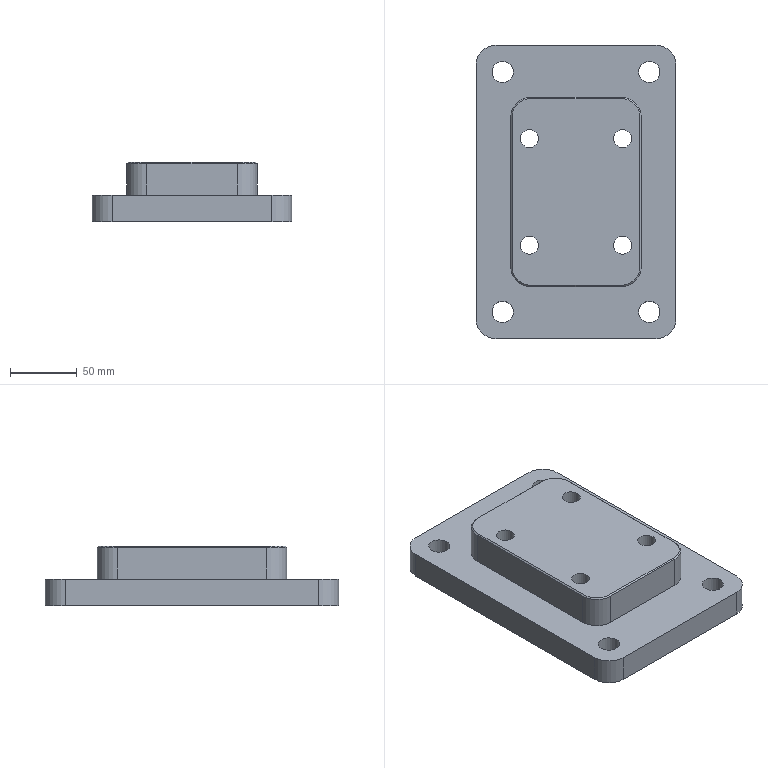NC program | NX | posted with a generic post | part box 150 x 220 x 45 mm
Lines 40 to 1292 of 5916:
(ZLEVEL_PROFILE_1_COPY , TOOL : D10)
N72 T10 M6
N74 G54
N76 G17 G0 G90 X91.61 Y82.1 S3200 M3
N78 G43 Z30. H10
N80 Z1.78
N82 G94 G1 Z-0.22 F2200.
N84 X92.478 Y80.599
N86 G3 X93.345 Y80.099 R1.
N88 G1 X94.677 Y80.1
N90 X95.
N92 G2 X115.1 Y60. R20.1
N94 G1 Y59.677
N96 Y58.345
N98 G3 X115.6 Y57.479 R1.
N100 G1 X117.1 Y56.612
N102 Z1.78
N104 G0 Z30.
N106 Z1.56
N108 G1 Z-0.44
N110 X115.6 Y57.479
N112 G2 X115.1 Y58.345 R1.
N114 G1 Y59.677
N116 Y60.
N118 G3 X95. Y80.1 R20.1
N120 G1 X94.677
N122 X93.345 Y80.099
N124 G2 X92.478 Y80.599 R1.
N126 G1 X91.61 Y82.1
N128 Z1.56
N130 G0 Z30.
N132 Z1.341
N134 G1 Z-0.659
N136 X92.478 Y80.599
N138 G3 X93.345 Y80.099 R1.
N140 G1 X94.677 Y80.1
N142 X95.
N144 G2 X115.1 Y60. R20.1
N146 G1 Y59.677
N148 Y58.345
N150 G3 X115.6 Y57.479 R1.
N152 G1 X117.1 Y56.612
N154 Z1.341
N156 G0 Z30.
N158 Z1.121
N160 G1 Z-0.879
N162 X115.6 Y57.479
N164 G2 X115.1 Y58.345 R1.
N166 G1 Y59.677
N168 Y60.
N170 G3 X95. Y80.1 R20.1
N172 G1 X94.677
N174 X93.345 Y80.099
N176 G2 X92.478 Y80.599 R1.
N178 G1 X91.61 Y82.1
N180 Z1.121
N182 G0 Z30.
N184 Z0.901
N186 G1 Z-1.099
N188 X92.478 Y80.599
N190 G3 X93.345 Y80.099 R1.
N192 G1 X94.677 Y80.1
N194 X95.
N196 G2 X115.1 Y60. R20.1
N198 G1 Y59.677
N200 Y58.345
N202 G3 X115.6 Y57.479 R1.
N204 G1 X117.1 Y56.612
N206 Z0.901
N208 G0 Z30.
N210 Z0.681
N212 G1 Z-1.319
N214 X115.6 Y57.479
N216 G2 X115.1 Y58.345 R1.
N218 G1 Y59.677
N220 Y60.
N222 G3 X95. Y80.1 R20.1
N224 G1 X94.677
N226 X93.345 Y80.099
N228 G2 X92.478 Y80.599 R1.
N230 G1 X91.61 Y82.1
N232 Z0.681
N234 G0 Z30.
N236 Z0.462
N238 G1 Z-1.538
N240 X92.478 Y80.599
N242 G3 X93.345 Y80.099 R1.
N244 G1 X94.677 Y80.1
N246 X95.
N248 G2 X115.1 Y60. R20.1
N250 G1 Y59.677
N252 Y58.345
N254 G3 X115.6 Y57.479 R1.
N256 G1 X117.1 Y56.612
N258 Z0.462
N260 G0 Z30.
N262 Z0.242
N264 G1 Z-1.758
N266 X115.6 Y57.479
N268 G2 X115.1 Y58.345 R1.
N270 G1 Y59.677
N272 Y60.
N274 G3 X95. Y80.1 R20.1
N276 G1 X94.677
N278 X93.345 Y80.099
N280 G2 X92.478 Y80.599 R1.
N282 G1 X91.61 Y82.1
N284 Z0.242
N286 G0 Z30.
N288 Z0.022
N290 G1 Z-1.978
N292 X92.478 Y80.599
N294 G3 X93.345 Y80.099 R1.
N296 G1 X94.677 Y80.1
N298 X95.
N300 G2 X115.1 Y60. R20.1
N302 G1 Y59.677
N304 Y58.345
N306 G3 X115.6 Y57.479 R1.
N308 G1 X117.1 Y56.612
N310 Z0.022
N312 G0 Z30.
N314 Z-0.198
N316 G1 Z-2.198
N318 X115.6 Y57.479
N320 G2 X115.1 Y58.345 R1.
N322 G1 Y59.677
N324 Y60.
N326 G3 X95. Y80.1 R20.1
N328 G1 X94.677
N330 X93.345 Y80.099
N332 G2 X92.478 Y80.599 R1.
N334 G1 X91.61 Y82.1
N336 Z-0.198
N338 G0 Z30.
N340 Z-0.418
N342 G1 Z-2.418
N344 X92.478 Y80.599
N346 G3 X93.345 Y80.099 R1.
N348 G1 X94.677 Y80.1
N350 X95.
N352 G2 X115.1 Y60. R20.1
N354 G1 Y59.677
N356 Y58.345
N358 G3 X115.6 Y57.479 R1.
N360 G1 X117.1 Y56.612
N362 Z-0.418
N364 G0 Z30.
N366 Z-0.637
N368 G1 Z-2.637
N370 X115.6 Y57.479
N372 G2 X115.1 Y58.345 R1.
N374 G1 Y59.677
N376 Y60.
N378 G3 X95. Y80.1 R20.1
N380 G1 X94.677
N382 X93.345 Y80.099
N384 G2 X92.478 Y80.599 R1.
N386 G1 X91.61 Y82.1
N388 Z-0.637
N390 G0 Z30.
N392 Z-0.857
N394 G1 Z-2.857
N396 X92.478 Y80.599
N398 G3 X93.345 Y80.099 R1.
N400 G1 X94.677 Y80.1
N402 X95.
N404 G2 X115.1 Y60. R20.1
N406 G1 Y59.677
N408 Y58.345
N410 G3 X115.6 Y57.479 R1.
N412 G1 X117.1 Y56.612
N414 Z-0.857
N416 G0 Z30.
N418 Z-1.077
N420 G1 Z-3.077
N422 X115.6 Y57.479
N424 G2 X115.1 Y58.345 R1.
N426 G1 Y59.677
N428 Y60.
N430 G3 X95. Y80.1 R20.1
N432 G1 X94.677
N434 X93.345 Y80.099
N436 G2 X92.478 Y80.599 R1.
N438 G1 X91.61 Y82.1
N440 Z-1.077
N442 G0 Z30.
N444 Z-1.297
N446 G1 Z-3.297
N448 X92.478 Y80.599
N450 G3 X93.345 Y80.099 R1.
N452 G1 X94.677 Y80.1
N454 X95.
N456 G2 X115.1 Y60. R20.1
N458 G1 Y59.677
N460 Y58.345
N462 G3 X115.6 Y57.479 R1.
N464 G1 X117.1 Y56.612
N466 Z-1.297
N468 G0 Z30.
N470 Z-1.516
N472 G1 Z-3.516
N474 X115.6 Y57.479
N476 G2 X115.1 Y58.345 R1.
N478 G1 Y59.677
N480 Y60.
N482 G3 X95. Y80.1 R20.1
N484 G1 X94.677
N486 X93.345 Y80.099
N488 G2 X92.478 Y80.599 R1.
N490 G1 X91.61 Y82.1
N492 Z-1.516
N494 G0 Z30.
N496 Z-1.736
N498 G1 Z-3.736
N500 X92.478 Y80.599
N502 G3 X93.345 Y80.099 R1.
N504 G1 X94.677 Y80.1
N506 X95.
N508 G2 X115.1 Y60. R20.1
N510 G1 Y59.677
N512 Y58.345
N514 G3 X115.6 Y57.479 R1.
N516 G1 X117.1 Y56.612
N518 Z-1.736
N520 G0 Z30.
N522 Z-1.956
N524 G1 Z-3.956
N526 X115.6 Y57.479
N528 G2 X115.1 Y58.345 R1.
N530 G1 Y59.677
N532 Y60.
N534 G3 X95. Y80.1 R20.1
N536 G1 X94.677
N538 X93.345 Y80.099
N540 G2 X92.478 Y80.599 R1.
N542 G1 X91.61 Y82.1
N544 Z-1.956
N546 G0 Z30.
N548 Z-2.176
N550 G1 Z-4.176
N552 X92.478 Y80.599
N554 G3 X93.345 Y80.099 R1.
N556 G1 X94.677 Y80.1
N558 X95.
N560 G2 X115.1 Y60. R20.1
N562 G1 Y59.677
N564 Y58.345
N566 G3 X115.6 Y57.479 R1.
N568 G1 X117.1 Y56.612
N570 Z-2.176
N572 G0 Z30.
N574 Z-2.396
N576 G1 Z-4.396
N578 X115.6 Y57.479
N580 G2 X115.1 Y58.345 R1.
N582 G1 Y59.677
N584 Y60.
N586 G3 X95. Y80.1 R20.1
N588 G1 X94.677
N590 X93.345 Y80.099
N592 G2 X92.478 Y80.599 R1.
N594 G1 X91.61 Y82.1
N596 Z-2.396
N598 G0 Z30.
N600 Z-2.615
N602 G1 Z-4.615
N604 X92.478 Y80.599
N606 G3 X93.345 Y80.099 R1.
N608 G1 X94.677 Y80.1
N610 X95.
N612 G2 X115.1 Y60. R20.1
N614 G1 Y59.677
N616 Y58.345
N618 G3 X115.6 Y57.479 R1.
N620 G1 X117.1 Y56.612
N622 Z-2.615
N624 G0 Z30.
N626 Z-2.835
N628 G1 Z-4.835
N630 X115.6 Y57.479
N632 G2 X115.1 Y58.345 R1.
N634 G1 Y59.677
N636 Y60.
N638 G3 X95. Y80.1 R20.1
N640 G1 X94.677
N642 X93.345 Y80.099
N644 G2 X92.478 Y80.599 R1.
N646 G1 X91.61 Y82.1
N648 Z-2.835
N650 G0 Z30.
N652 Z-3.055
N654 G1 Z-5.055
N656 X92.478 Y80.599
N658 G3 X93.345 Y80.099 R1.
N660 G1 X94.677 Y80.1
N662 X95.
N664 G2 X115.1 Y60. R20.1
N666 G1 Y59.677
N668 Y58.345
N670 G3 X115.6 Y57.479 R1.
N672 G1 X117.1 Y56.612
N674 Z-3.055
N676 G0 Z30.
N678 Z-3.275
N680 G1 Z-5.275
N682 X115.6 Y57.479
N684 G2 X115.1 Y58.345 R1.
N686 G1 Y59.677
N688 Y60.
N690 G3 X95. Y80.1 R20.1
N692 G1 X94.677
N694 X93.345 Y80.099
N696 G2 X92.478 Y80.599 R1.
N698 G1 X91.61 Y82.1
N700 Z-3.275
N702 G0 Z30.
N704 Z-3.495
N706 G1 Z-5.495
N708 X92.478 Y80.599
N710 G3 X93.345 Y80.099 R1.
N712 G1 X94.677 Y80.1
N714 X95.
N716 G2 X115.1 Y60. R20.1
N718 G1 Y59.677
N720 Y58.345
N722 G3 X115.6 Y57.479 R1.
N724 G1 X117.1 Y56.612
N726 Z-3.495
N728 G0 Z30.
N730 Z-3.714
N732 G1 Z-5.714
N734 X115.6 Y57.479
N736 G2 X115.1 Y58.345 R1.
N738 G1 Y59.677
N740 Y60.
N742 G3 X95. Y80.1 R20.1
N744 G1 X94.677
N746 X93.345 Y80.099
N748 G2 X92.478 Y80.599 R1.
N750 G1 X91.61 Y82.1
N752 Z-3.714
N754 G0 Z30.
N756 Z-3.934
N758 G1 Z-5.934
N760 X92.478 Y80.599
N762 G3 X93.345 Y80.099 R1.
N764 G1 X94.677 Y80.1
N766 X95.
N768 G2 X115.1 Y60. R20.1
N770 G1 Y59.677
N772 Y58.345
N774 G3 X115.6 Y57.479 R1.
N776 G1 X117.1 Y56.612
N778 Z-3.934
N780 G0 Z30.
N782 Z-4.154
N784 G1 Z-6.154
N786 X115.6 Y57.479
N788 G2 X115.1 Y58.345 R1.
N790 G1 Y59.677
N792 Y60.
N794 G3 X95. Y80.1 R20.1
N796 G1 X94.677
N798 X93.345 Y80.099
N800 G2 X92.478 Y80.599 R1.
N802 G1 X91.61 Y82.1
N804 Z-4.154
N806 G0 Z30.
N808 Z-4.374
N810 G1 Z-6.374
N812 X92.478 Y80.599
N814 G3 X93.345 Y80.099 R1.
N816 G1 X94.677 Y80.1
N818 X95.
N820 G2 X115.1 Y60. R20.1
N822 G1 Y59.677
N824 Y58.345
N826 G3 X115.6 Y57.479 R1.
N828 G1 X117.1 Y56.612
N830 Z-4.374
N832 G0 Z30.
N834 Z-4.593
N836 G1 Z-6.593
N838 X115.6 Y57.479
N840 G2 X115.1 Y58.345 R1.
N842 G1 Y59.677
N844 Y60.
N846 G3 X95. Y80.1 R20.1
N848 G1 X94.677
N850 X93.345 Y80.099
N852 G2 X92.478 Y80.599 R1.
N854 G1 X91.61 Y82.1
N856 Z-4.593
N858 G0 Z30.
N860 Z-4.813
N862 G1 Z-6.813
N864 X92.478 Y80.599
N866 G3 X93.345 Y80.099 R1.
N868 G1 X94.677 Y80.1
N870 X95.
N872 G2 X115.1 Y60. R20.1
N874 G1 Y59.677
N876 Y58.345
N878 G3 X115.6 Y57.479 R1.
N880 G1 X117.1 Y56.612
N882 Z-4.813
N884 G0 Z30.
N886 Z-5.033
N888 G1 Z-7.033
N890 X115.6 Y57.479
N892 G2 X115.1 Y58.345 R1.
N894 G1 Y59.677
N896 Y60.
N898 G3 X95. Y80.1 R20.1
N900 G1 X94.677
N902 X93.345 Y80.099
N904 G2 X92.478 Y80.599 R1.
N906 G1 X91.61 Y82.1
N908 Z-5.033
N910 G0 Z30.
N912 Z-5.253
N914 G1 Z-7.253
N916 X92.478 Y80.599
N918 G3 X93.345 Y80.099 R1.
N920 G1 X94.677 Y80.1
N922 X95.
N924 G2 X115.1 Y60. R20.1
N926 G1 Y59.677
N928 Y58.345
N930 G3 X115.6 Y57.479 R1.
N932 G1 X117.1 Y56.612
N934 Z-5.253
N936 G0 Z30.
N938 Z-5.473
N940 G1 Z-7.473
N942 X115.6 Y57.479
N944 G2 X115.1 Y58.345 R1.
N946 G1 Y59.677
N948 Y60.
N950 G3 X95. Y80.1 R20.1
N952 G1 X94.677
N954 X93.345 Y80.099
N956 G2 X92.478 Y80.599 R1.
N958 G1 X91.61 Y82.1
N960 Z-5.473
N962 G0 Z30.
N964 Z-5.692
N966 G1 Z-7.692
N968 X92.478 Y80.599
N970 G3 X93.345 Y80.099 R1.
N972 G1 X94.677 Y80.1
N974 X95.
N976 G2 X115.1 Y60. R20.1
N978 G1 Y59.677
N980 Y58.345
N982 G3 X115.6 Y57.479 R1.
N984 G1 X117.1 Y56.612
N986 Z-5.692
N988 G0 Z30.
N990 Z-5.912
N992 G1 Z-7.912
N994 X115.6 Y57.479
N996 G2 X115.1 Y58.345 R1.
N998 G1 Y59.677
N1000 Y60.
N1002 G3 X95. Y80.1 R20.1
N1004 G1 X94.677
N1006 X93.345 Y80.099
N1008 G2 X92.478 Y80.599 R1.
N1010 G1 X91.61 Y82.1
N1012 Z-5.912
N1014 G0 Z30.
N1016 Z-6.132
N1018 G1 Z-8.132
N1020 X92.478 Y80.599
N1022 G3 X93.345 Y80.099 R1.
N1024 G1 X94.677 Y80.1
N1026 X95.
N1028 G2 X115.1 Y60. R20.1
N1030 G1 Y59.677
N1032 Y58.345
N1034 G3 X115.6 Y57.479 R1.
N1036 G1 X117.1 Y56.612
N1038 Z-6.132
N1040 G0 Z30.
N1042 Z-6.352
N1044 G1 Z-8.352
N1046 X115.6 Y57.479
N1048 G2 X115.1 Y58.345 R1.
N1050 G1 Y59.677
N1052 Y60.
N1054 G3 X95. Y80.1 R20.1
N1056 G1 X94.677
N1058 X93.345 Y80.099
N1060 G2 X92.478 Y80.599 R1.
N1062 G1 X91.61 Y82.1
N1064 Z-6.352
N1066 G0 Z30.
N1068 Z-6.571
N1070 G1 Z-8.571
N1072 X92.478 Y80.599
N1074 G3 X93.345 Y80.099 R1.
N1076 G1 X94.677 Y80.1
N1078 X95.
N1080 G2 X115.1 Y60. R20.1
N1082 G1 Y59.677
N1084 Y58.345
N1086 G3 X115.6 Y57.479 R1.
N1088 G1 X117.1 Y56.612
N1090 Z-6.571
N1092 G0 Z30.
N1094 Z-6.791
N1096 G1 Z-8.791
N1098 X115.6 Y57.479
N1100 G2 X115.1 Y58.345 R1.
N1102 G1 Y59.677
N1104 Y60.
N1106 G3 X95. Y80.1 R20.1
N1108 G1 X94.677
N1110 X93.345 Y80.099
N1112 G2 X92.478 Y80.599 R1.
N1114 G1 X91.61 Y82.1
N1116 Z-6.791
N1118 G0 Z30.
N1120 Z-7.011
N1122 G1 Z-9.011
N1124 X92.478 Y80.599
N1126 G3 X93.345 Y80.099 R1.
N1128 G1 X94.677 Y80.1
N1130 X95.
N1132 G2 X115.1 Y60. R20.1
N1134 G1 Y59.677
N1136 Y58.345
N1138 G3 X115.6 Y57.479 R1.
N1140 G1 X117.1 Y56.612
N1142 Z-7.011
N1144 G0 Z30.
N1146 Z-7.231
N1148 G1 Z-9.231
N1150 X115.6 Y57.479
N1152 G2 X115.1 Y58.345 R1.
N1154 G1 Y59.677
N1156 Y60.
N1158 G3 X95. Y80.1 R20.1
N1160 G1 X94.677
N1162 X93.345 Y80.099
N1164 G2 X92.478 Y80.599 R1.
N1166 G1 X91.61 Y82.1
N1168 Z-7.231
N1170 G0 Z30.
N1172 Z-7.451
N1174 G1 Z-9.451
N1176 X92.478 Y80.599
N1178 G3 X93.345 Y80.099 R1.
N1180 G1 X94.677 Y80.1
N1182 X95.
N1184 G2 X115.1 Y60. R20.1
N1186 G1 Y59.677
N1188 Y58.345
N1190 G3 X115.6 Y57.479 R1.
N1192 G1 X117.1 Y56.612
N1194 Z-7.451
N1196 G0 Z30.
N1198 Z-7.67
N1200 G1 Z-9.67
N1202 X115.6 Y57.479
N1204 G2 X115.1 Y58.345 R1.
N1206 G1 Y59.677
N1208 Y60.
N1210 G3 X95. Y80.1 R20.1
N1212 G1 X94.677
N1214 X93.345 Y80.099
N1216 G2 X92.478 Y80.599 R1.
N1218 G1 X91.61 Y82.1
N1220 Z-7.67
N1222 G0 Z30.
N1224 Z-7.89
N1226 G1 Z-9.89
N1228 X92.478 Y80.599
N1230 G3 X93.345 Y80.099 R1.
N1232 G1 X94.677 Y80.1
N1234 X95.
N1236 G2 X115.1 Y60. R20.1
N1238 G1 Y59.677
N1240 Y58.345
N1242 G3 X115.6 Y57.479 R1.
N1244 G1 X117.1 Y56.612
N1246 Z-7.89
N1248 G0 Z30.
N1250 Z-8.11
N1252 G1 Z-10.11
N1254 X115.6 Y57.479
N1256 G2 X115.1 Y58.345 R1.
N1258 G1 Y59.677
N1260 Y60.
N1262 G3 X95. Y80.1 R20.1
N1264 G1 X94.677
N1266 X93.345 Y80.099
N1268 G2 X92.478 Y80.599 R1.
N1270 G1 X91.61 Y82.1
N1272 Z-8.11
N1274 G0 Z30.
N1276 X91.611 Z-8.33
N1278 G1 Z-10.33
N1280 X92.478 Y80.599
N1282 G3 X93.345 Y80.099 R1.
N1284 G1 X94.677 Y80.1
N1286 X95.
N1288 G2 X115.1 Y60. R20.1
N1290 G1 Y59.677
N1292 Y58.345
N1294 G3 X115.6 Y57.479 R1.
N1296 G1 X117.1 Y56.612
N1298 Z-8.33
N1300 G0 Z30.
N1302 Z-8.549
N1304 G1 Z-10.549
N1306 X115.6 Y57.479
N1308 G2 X115.1 Y58.345 R1.
N1310 G1 Y59.677
N1312 Y60.
N1314 G3 X95. Y80.1 R20.1
N1316 G1 X94.677
N1318 X93.345 Y80.099
N1320 G2 X92.478 Y80.599 R1.
N1322 G1 X91.611 Y82.1
N1324 Z-8.549
N1326 G0 Z30.
N1328 Z-8.769
N1330 G1 Z-10.769
N1332 X92.478 Y80.599
N1334 G3 X93.345 Y80.099 R1.
N1336 G1 X94.677 Y80.1
N1338 X95.
N1340 G2 X115.1 Y60. R20.1
N1342 G1 Y59.677
N1344 Y58.345
N1346 G3 X115.6 Y57.479 R1.
N1348 G1 X117.1 Y56.612
N1350 Z-8.769
N1352 G0 Z30.
N1354 Z-8.989
N1356 G1 Z-10.989
N1358 X115.6 Y57.479
N1360 G2 X115.1 Y58.345 R1.
N1362 G1 Y59.677
N1364 Y60.
N1366 G3 X95. Y80.1 R20.1
N1368 G1 X94.677
N1370 X93.345 Y80.099
N1372 G2 X92.478 Y80.599 R1.
N1374 G1 X91.611 Y82.1
N1376 Z-8.989
N1378 G0 Z30.
N1380 Z-9.209
N1382 G1 Z-11.209
N1384 X92.478 Y80.599
N1386 G3 X93.345 Y80.099 R1.
N1388 G1 X94.677 Y80.1
N1390 X95.
N1392 G2 X115.1 Y60. R20.1
N1394 G1 Y59.677
N1396 Y58.345
N1398 G3 X115.6 Y57.479 R1.
N1400 G1 X117.1 Y56.612
N1402 Z-9.209
N1404 G0 Z30.
N1406 Z-9.429
N1408 G1 Z-11.429
N1410 X115.6 Y57.479
N1412 G2 X115.1 Y58.345 R1.
N1414 G1 Y59.677
N1416 Y60.
N1418 G3 X95. Y80.1 R20.1
N1420 G1 X94.677
N1422 X93.345 Y80.099
N1424 G2 X92.478 Y80.599 R1.
N1426 G1 X91.611 Y82.1
N1428 Z-9.429
N1430 G0 Z30.
N1432 Z-9.648
N1434 G1 Z-11.648
N1436 X92.478 Y80.599
N1438 G3 X93.345 Y80.099 R1.
N1440 G1 X94.677 Y80.1
N1442 X95.
N1444 G2 X115.1 Y60. R20.1
N1446 G1 Y59.677
N1448 Y58.345
N1450 G3 X115.6 Y57.479 R1.
N1452 G1 X117.1 Y56.612
N1454 Z-9.648
N1456 G0 Z30.
N1458 Z-9.868
N1460 G1 Z-11.868
N1462 X115.6 Y57.479
N1464 G2 X115.1 Y58.345 R1.
N1466 G1 Y59.677
N1468 Y60.
N1470 G3 X95. Y80.1 R20.1
N1472 G1 X94.677
N1474 X93.345 Y80.099
N1476 G2 X92.478 Y80.599 R1.
N1478 G1 X91.611 Y82.1
N1480 Z-9.868
N1482 G0 Z30.
N1484 Z-10.088
N1486 G1 Z-12.088
N1488 X92.478 Y80.599
N1490 G3 X93.345 Y80.099 R1.
N1492 G1 X94.677 Y80.1
N1494 X95.
N1496 G2 X115.1 Y60. R20.1
N1498 G1 Y59.677
N1500 Y58.345
N1502 G3 X115.6 Y57.479 R1.
N1504 G1 X117.1 Y56.612
N1506 Z-10.088
N1508 G0 Z30.
N1510 Z-10.308
N1512 G1 Z-12.308
N1514 X115.6 Y57.479
N1516 G2 X115.1 Y58.345 R1.
N1518 G1 Y59.677
N1520 Y60.
N1522 G3 X95. Y80.1 R20.1
N1524 G1 X94.677
N1526 X93.345 Y80.099
N1528 G2 X92.478 Y80.599 R1.
N1530 G1 X91.611 Y82.1
N1532 Z-10.308
N1534 G0 Z30.
N1536 Z-10.527
N1538 G1 Z-12.527
N1540 X92.478 Y80.599
N1542 G3 X93.345 Y80.099 R1.
N1544 G1 X94.677 Y80.1
N1546 X95.
N1548 G2 X115.1 Y60. R20.1
N1550 G1 Y59.677
N1552 Y58.345
N1554 G3 X115.6 Y57.479 R1.
N1556 G1 X117.1 Y56.612
N1558 Z-10.527
N1560 G0 Z30.
N1562 Z-10.747
N1564 G1 Z-12.747
N1566 X115.6 Y57.479
N1568 G2 X115.1 Y58.345 R1.
N1570 G1 Y59.677
N1572 Y60.
N1574 G3 X95. Y80.1 R20.1
N1576 G1 X94.677
N1578 X93.345 Y80.099
N1580 G2 X92.478 Y80.599 R1.
N1582 G1 X91.611 Y82.1
N1584 Z-10.747
N1586 G0 Z30.
N1588 Z-10.967
N1590 G1 Z-12.967
N1592 X92.478 Y80.599
N1594 G3 X93.345 Y80.099 R1.
N1596 G1 X94.677 Y80.1
N1598 X95.
N1600 G2 X115.1 Y60. R20.1
N1602 G1 Y59.677
N1604 Y58.345
N1606 G3 X115.6 Y57.479 R1.
N1608 G1 X117.1 Y56.612
N1610 Z-10.967
N1612 G0 Z30.
N1614 Z-11.187
N1616 G1 Z-13.187
N1618 X115.6 Y57.479
N1620 G2 X115.1 Y58.345 R1.
N1622 G1 Y59.677
N1624 Y60.
N1626 G3 X95. Y80.1 R20.1
N1628 G1 X94.677
N1630 X93.345 Y80.099
N1632 G2 X92.478 Y80.599 R1.
N1634 G1 X91.611 Y82.1
N1636 Z-11.187
N1638 G0 Z30.
N1640 Z-11.407
N1642 G1 Z-13.407
N1644 X92.478 Y80.599
N1646 G3 X93.345 Y80.099 R1.
N1648 G1 X94.677 Y80.1
N1650 X95.
N1652 G2 X115.1 Y60. R20.1
N1654 G1 Y59.677
N1656 Y58.345
N1658 G3 X115.6 Y57.479 R1.
N1660 G1 X117.1 Y56.612
N1662 Z-11.407
N1664 G0 Z30.
N1666 Z-11.626
N1668 G1 Z-13.626
N1670 X115.6 Y57.479
N1672 G2 X115.1 Y58.345 R1.
N1674 G1 Y59.677
N1676 Y60.
N1678 G3 X95. Y80.1 R20.1
N1680 G1 X94.677
N1682 X93.345 Y80.099
N1684 G2 X92.478 Y80.599 R1.
N1686 G1 X91.611 Y82.1
N1688 Z-11.626
N1690 G0 Z30.
N1692 Z-11.846
N1694 G1 Z-13.846
N1696 X92.478 Y80.599
N1698 G3 X93.345 Y80.099 R1.
N1700 G1 X94.677 Y80.1
N1702 X95.
N1704 G2 X115.1 Y60. R20.1
N1706 G1 Y59.677
N1708 Y58.345
N1710 G3 X115.6 Y57.479 R1.
N1712 G1 X117.1 Y56.612
N1714 Z-11.846
N1716 G0 Z30.
N1718 Z-12.066
N1720 G1 Z-14.066
N1722 X115.6 Y57.479
N1724 G2 X115.1 Y58.345 R1.
N1726 G1 Y59.677
N1728 Y60.
N1730 G3 X95. Y80.1 R20.1
N1732 G1 X94.677
N1734 X93.345 Y80.099
N1736 G2 X92.478 Y80.599 R1.
N1738 G1 X91.611 Y82.1
N1740 Z-12.066
N1742 G0 Z30.
N1744 Z-12.286
N1746 G1 Z-14.286
N1748 X92.478 Y80.599
N1750 G3 X93.345 Y80.099 R1.
N1752 G1 X94.677 Y80.1
N1754 X95.
N1756 G2 X115.1 Y60. R20.1
N1758 G1 Y59.677
N1760 Y58.345
N1762 G3 X115.6 Y57.479 R1.
N1764 G1 X117.1 Y56.612
N1766 Z-12.286
N1768 G0 Z30.
N1770 Z-12.505
N1772 G1 Z-14.505
N1774 X115.6 Y57.479
N1776 G2 X115.1 Y58.345 R1.
N1778 G1 Y59.677
N1780 Y60.
N1782 G3 X95. Y80.1 R20.1
N1784 G1 X94.677
N1786 X93.345 Y80.099
N1788 G2 X92.478 Y80.599 R1.
N1790 G1 X91.611 Y82.1
N1792 Z-12.505
N1794 G0 Z30.
N1796 Z-12.725
N1798 G1 Z-14.725
N1800 X92.478 Y80.599
N1802 G3 X93.345 Y80.099 R1.
N1804 G1 X94.677 Y80.1
N1806 X95.
N1808 G2 X115.1 Y60. R20.1
N1810 G1 Y59.677
N1812 Y58.345
N1814 G3 X115.6 Y57.479 R1.
N1816 G1 X117.1 Y56.612
N1818 Z-12.725
N1820 G0 Z30.
N1822 Y56.613 Z-12.945
N1824 G1 Z-14.945
N1826 X115.6 Y57.479
N1828 G2 X115.1 Y58.345 R1.
N1830 G1 Y59.677
N1832 Y60.
N1834 G3 X95. Y80.1 R20.1
N1836 G1 X94.677
N1838 X93.345 Y80.099
N1840 G2 X92.478 Y80.599 R1.
N1842 G1 X91.611 Y82.1
N1844 Z-12.945
N1846 G0 Z30.
N1848 Z-13.165
N1850 G1 Z-15.165
N1852 X92.478 Y80.599
N1854 G3 X93.345 Y80.099 R1.
N1856 G1 X94.677 Y80.1
N1858 X95.
N1860 G2 X115.1 Y60. R20.1
N1862 G1 Y59.677
N1864 Y58.345
N1866 G3 X115.6 Y57.479 R1.
N1868 G1 X117.1 Y56.613
N1870 Z-13.165
N1872 G0 Z30.
N1874 Z-13.385
N1876 G1 Z-15.385
N1878 X115.6 Y57.479
N1880 G2 X115.1 Y58.345 R1.
N1882 G1 Y59.677
N1884 Y60.
N1886 G3 X95. Y80.1 R20.1
N1888 G1 X94.677
N1890 X93.345 Y80.099
N1892 G2 X92.478 Y80.599 R1.
N1894 G1 X91.611 Y82.1
N1896 Z-13.385
N1898 G0 Z30.
N1900 Z-13.604
N1902 G1 Z-15.604
N1904 X92.478 Y80.599
N1906 G3 X93.345 Y80.099 R1.
N1908 G1 X94.677 Y80.1
N1910 X95.
N1912 G2 X115.1 Y60. R20.1
N1914 G1 Y59.677
N1916 Y58.345
N1918 G3 X115.6 Y57.479 R1.
N1920 G1 X117.1 Y56.613
N1922 Z-13.604
N1924 G0 Z30.
N1926 Z-13.824
N1928 G1 Z-15.824
N1930 X115.6 Y57.479
N1932 G2 X115.1 Y58.345 R1.
N1934 G1 Y59.677
N1936 Y60.
N1938 G3 X95. Y80.1 R20.1
N1940 G1 X94.677
N1942 X93.345 Y80.099
N1944 G2 X92.478 Y80.599 R1.
N1946 G1 X91.611 Y82.1
N1948 Z-13.824
N1950 G0 Z30.
N1952 Z-14.044
N1954 G1 Z-16.044
N1956 X92.478 Y80.599
N1958 G3 X93.345 Y80.099 R1.
N1960 G1 X94.677 Y80.1
N1962 X95.
N1964 G2 X115.1 Y60. R20.1
N1966 G1 Y59.677
N1968 Y58.345
N1970 G3 X115.6 Y57.479 R1.
N1972 G1 X117.1 Y56.613
N1974 Z-14.044
N1976 G0 Z30.
N1978 Z-14.264
N1980 G1 Z-16.264
N1982 X115.6 Y57.479
N1984 G2 X115.1 Y58.345 R1.
N1986 G1 Y59.677
N1988 Y60.
N1990 G3 X95. Y80.1 R20.1
N1992 G1 X94.677
N1994 X93.345 Y80.099
N1996 G2 X92.478 Y80.599 R1.
N1998 G1 X91.611 Y82.1
N2000 Z-14.264
N2002 G0 Z30.
N2004 Z-14.484
N2006 G1 Z-16.484
N2008 X92.478 Y80.599
N2010 G3 X93.345 Y80.099 R1.
N2012 G1 X94.677 Y80.1
N2014 X95.
N2016 G2 X115.1 Y60. R20.1
N2018 G1 Y59.677
N2020 Y58.345
N2022 G3 X115.6 Y57.479 R1.
N2024 G1 X117.1 Y56.613
N2026 Z-14.484
N2028 G0 Z30.
N2030 Z-14.703
N2032 G1 Z-16.703
N2034 X115.6 Y57.479
N2036 G2 X115.1 Y58.345 R1.
N2038 G1 Y59.677
N2040 Y60.
N2042 G3 X95. Y80.1 R20.1
N2044 G1 X94.677
N2046 X93.345 Y80.099
N2048 G2 X92.478 Y80.599 R1.
N2050 G1 X91.611 Y82.1
N2052 Z-14.703
N2054 G0 Z30.
N2056 Z-14.923
N2058 G1 Z-16.923
N2060 X92.478 Y80.599
N2062 G3 X93.345 Y80.099 R1.
N2064 G1 X94.677 Y80.1
N2066 X95.
N2068 G2 X115.1 Y60. R20.1
N2070 G1 Y59.677
N2072 Y58.345
N2074 G3 X115.6 Y57.479 R1.
N2076 G1 X117.1 Y56.613
N2078 Z-14.923
N2080 G0 Z30.
N2082 Z-15.143
N2084 G1 Z-17.143
N2086 X115.6 Y57.479
N2088 G2 X115.1 Y58.345 R1.
N2090 G1 Y59.677
N2092 Y60.
N2094 G3 X95. Y80.1 R20.1
N2096 G1 X94.677
N2098 X93.345 Y80.099
N2100 G2 X92.478 Y80.599 R1.
N2102 G1 X91.611 Y82.1
N2104 Z-15.143
N2106 G0 Z30.
N2108 Z-15.363
N2110 G1 Z-17.363
N2112 X92.478 Y80.599
N2114 G3 X93.345 Y80.099 R1.
N2116 G1 X94.677 Y80.1
N2118 X95.
N2120 G2 X115.1 Y60. R20.1
N2122 G1 Y59.677
N2124 Y58.345
N2126 G3 X115.6 Y57.479 R1.
N2128 G1 X117.1 Y56.613
N2130 Z-15.363
N2132 G0 Z30.
N2134 Z-15.582
N2136 G1 Z-17.582
N2138 X115.6 Y57.479
N2140 G2 X115.1 Y58.345 R1.
N2142 G1 Y59.677
N2144 Y60.
N2146 G3 X95. Y80.1 R20.1
N2148 G1 X94.677
N2150 X93.345 Y80.099
N2152 G2 X92.478 Y80.599 R1.
N2154 G1 X91.611 Y82.1
N2156 Z-15.582
N2158 G0 Z30.
N2160 Z-15.802
N2162 G1 Z-17.802
N2164 X92.478 Y80.599
N2166 G3 X93.345 Y80.099 R1.
N2168 G1 X94.677 Y80.1
N2170 X95.
N2172 G2 X115.1 Y60. R20.1
N2174 G1 Y59.677
N2176 Y58.345
N2178 G3 X115.6 Y57.479 R1.
N2180 G1 X117.1 Y56.613
N2182 Z-15.802
N2184 G0 Z30.
N2186 Z-16.022
N2188 G1 Z-18.022
N2190 X115.6 Y57.479
N2192 G2 X115.1 Y58.345 R1.
N2194 G1 Y59.677
N2196 Y60.
N2198 G3 X95. Y80.1 R20.1
N2200 G1 X94.677
N2202 X93.345 Y80.099
N2204 G2 X92.478 Y80.599 R1.
N2206 G1 X91.611 Y82.1
N2208 Z-16.022
N2210 G0 Z30.
N2212 Z-16.242
N2214 G1 Z-18.242
N2216 X92.478 Y80.599
N2218 G3 X93.345 Y80.099 R1.
N2220 G1 X94.677 Y80.1
N2222 X95.
N2224 G2 X115.1 Y60. R20.1
N2226 G1 Y59.677
N2228 Y58.345
N2230 G3 X115.6 Y57.479 R1.
N2232 G1 X117.1 Y56.613
N2234 Z-16.242
N2236 G0 Z30.
N2238 Z-16.462
N2240 G1 Z-18.462
N2242 X115.6 Y57.479
N2244 G2 X115.1 Y58.345 R1.
N2246 G1 Y59.677
N2248 Y60.
N2250 G3 X95. Y80.1 R20.1
N2252 G1 X94.677
N2254 X93.345 Y80.099
N2256 G2 X92.478 Y80.599 R1.
N2258 G1 X91.611 Y82.1
N2260 Z-16.462
N2262 G0 Z30.
N2264 Z-16.681
N2266 G1 Z-18.681
N2268 X92.478 Y80.599
N2270 G3 X93.345 Y80.099 R1.
N2272 G1 X94.677 Y80.1
N2274 X95.
N2276 G2 X115.1 Y60. R20.1
N2278 G1 Y59.677
N2280 Y58.345
N2282 G3 X115.6 Y57.479 R1.
N2284 G1 X117.1 Y56.613
N2286 Z-16.681
N2288 G0 Z30.
N2290 Z-16.901
N2292 G1 Z-18.901
N2294 X115.6 Y57.479
N2296 G2 X115.1 Y58.345 R1.
N2298 G1 Y59.677
N2300 Y60.
N2302 G3 X95. Y80.1 R20.1
N2304 G1 X94.677
N2306 X93.345 Y80.099
N2308 G2 X92.478 Y80.599 R1.
N2310 G1 X91.611 Y82.1
N2312 Z-16.901
N2314 G0 Z30.
N2316 Z-17.121
N2318 G1 Z-19.121
N2320 X92.478 Y80.599
N2322 G3 X93.345 Y80.099 R1.
N2324 G1 X94.677 Y80.1
N2326 X95.
N2328 G2 X115.1 Y60. R20.1
N2330 G1 Y59.677
N2332 Y58.345
N2334 G3 X115.6 Y57.479 R1.
N2336 G1 X117.1 Y56.613
N2338 Z-17.121
N2340 G0 Z30.
N2342 Z-17.341
N2344 G1 Z-19.341
N2346 X115.6 Y57.479
N2348 G2 X115.1 Y58.345 R1.
N2350 G1 Y59.677
N2352 Y60.
N2354 G3 X95. Y80.1 R20.1
N2356 G1 X94.677
N2358 X93.345 Y80.099
N2360 G2 X92.478 Y80.599 R1.
N2362 G1 X91.611 Y82.1
N2364 Z-17.341
N2366 G0 Z30.
N2368 Z-17.56
N2370 G1 Z-19.56
N2372 X92.478 Y80.599
N2374 G3 X93.345 Y80.099 R1.
N2376 G1 X94.677 Y80.1
N2378 X95.
N2380 G2 X115.1 Y60. R20.1
N2382 G1 Y59.677
N2384 Y58.345
N2386 G3 X115.6 Y57.479 R1.
N2388 G1 X117.1 Y56.613
N2390 Z-17.56
N2392 G0 Z30.
N2394 Z-17.78
N2396 G1 Z-19.78
N2398 X115.6 Y57.479
N2400 G2 X115.1 Y58.345 R1.
N2402 G1 Y59.677
N2404 Y60.
N2406 G3 X95. Y80.1 R20.1
N2408 G1 X94.677
N2410 X93.345 Y80.099
N2412 G2 X92.478 Y80.599 R1.
N2414 G1 X91.611 Y82.1
N2416 Z-17.78
N2418 G0 Z30.
N2420 Z-18.
N2422 G1 Z-20.
N2424 X92.478 Y80.599
N2426 G3 X93.345 Y80.099 R1.
N2428 G1 X94.677 Y80.1
N2430 X95.
N2432 G2 X115.1 Y60. R20.1
N2434 G1 Y59.677
N2436 Y58.345
N2438 G3 X115.6 Y57.479 R1.
N2440 G1 X117.1 Y56.613
N2442 Z-18.
N2444 G0 Z30.
N2446 Y-56.612
N2448 Z1.78
N2450 G1 Z-0.22
N2452 X115.6 Y-57.479
N2454 G3 X115.1 Y-58.345 R1.
N2456 G1 Y-59.677
N2458 Y-60.
N2460 G2 X95. Y-80.1 R20.1
N2462 G1 X94.677
N2464 X93.345
N2466 G3 X92.479 Y-80.6 R1.
N2468 G1 X91.612 Y-82.1
N2470 Z1.78
N2472 G0 Z30.
N2474 Z1.56
N2476 G1 Z-0.44
N2478 X92.479 Y-80.6
N2480 G2 X93.345 Y-80.1 R1.
N2482 G1 X94.677
N2484 X95.
N2486 G3 X115.1 Y-60. R20.1
N2488 G1 Y-59.677
N2490 Y-58.345
N2492 G2 X115.6 Y-57.479 R1.
N2494 G1 X117.1 Y-56.612
N2496 Z1.56
N2498 G0 Z30.
N2500 Z1.341
N2502 G1 Z-0.659
N2504 X115.6 Y-57.479
N2506 G3 X115.1 Y-58.345 R1.
N2508 G1 Y-59.677
N2510 Y-60.
N2512 G2 X95. Y-80.1 R20.1
N2514 G1 X94.677
N2516 X93.345
N2518 G3 X92.479 Y-80.6 R1.
N2520 G1 X91.612 Y-82.1
N2522 Z1.341
N2524 G0 Z30.
N2526 Z1.121
N2528 G1 Z-0.879
N2530 X92.479 Y-80.6
N2532 G2 X93.345 Y-80.1 R1.
N2534 G1 X94.677
N2536 X95.
N2538 G3 X115.1 Y-60. R20.1
N2540 G1 Y-59.677
N2542 Y-58.345
N2544 G2 X115.6 Y-57.479 R1.
N2546 G1 X117.1 Y-56.612
N2548 Z1.121
N2550 G0 Z30.
N2552 Z0.901
N2554 G1 Z-1.099
N2556 X115.6 Y-57.479
N2558 G3 X115.1 Y-58.345 R1.
N2560 G1 Y-59.677
N2562 Y-60.
N2564 G2 X95. Y-80.1 R20.1
N2566 G1 X94.677
N2568 X93.345
N2570 G3 X92.479 Y-80.6 R1.